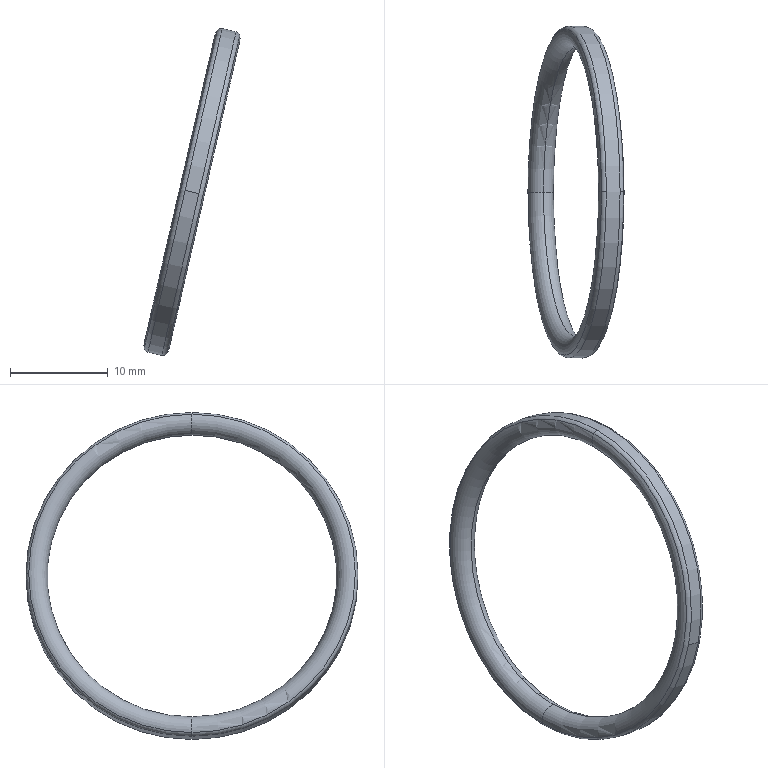Part | SolidWorks | features BaseBody 1 | 1 solid | 12 faces | box 9.855 x 34.04 x 33.526 mm | volume 478.172 mm3 | torus 10 | cylinder 2 | commonest cylinder face diameters 34.04 x2
STEP:
#1=CARTESIAN_POINT('',(1966.289,-176.,834.72));
#2=VERTEX_POINT('',#1);
#3=CARTESIAN_POINT('',(1964.722,-176.,833.139));
#4=VERTEX_POINT('',#3);
#5=CARTESIAN_POINT('',(1965.996,-176.,833.443));
#6=DIRECTION('',(0.,-1.,0.));
#7=DIRECTION('',(0.7736,0.,-0.6337));
#8=AXIS2_PLACEMENT_3D('',#5,#6,#7);
#9=CIRCLE('',#8,1.31);
#10=EDGE_CURVE('',#2,#4,#9,.T.);
#11=ORIENTED_EDGE('',*,*,#10,.F.);
#12=CARTESIAN_POINT('',(1972.938,-176.,863.666));
#13=VERTEX_POINT('',#12);
#14=CARTESIAN_POINT('',(1969.614,-176.,849.193));
#15=DIRECTION('',(0.9746,0.,-0.2239));
#16=DIRECTION('',(-0.2239,0.,-0.9746));
#17=AXIS2_PLACEMENT_3D('',#14,#15,#16);
#18=CIRCLE('',#17,14.85);
#19=EDGE_CURVE('',#2,#13,#18,.T.);
#20=ORIENTED_EDGE('',*,*,#19,.T.);
#21=CARTESIAN_POINT('',(1972.218,-176.,865.773));
#22=VERTEX_POINT('',#21);
#23=CARTESIAN_POINT('',(1973.231,-176.,864.943));
#24=DIRECTION('',(0.,-1.,0.));
#25=DIRECTION('',(-0.7736,0.,0.6337));
#26=AXIS2_PLACEMENT_3D('',#23,#24,#25);
#27=CIRCLE('',#26,1.31);
#28=EDGE_CURVE('',#22,#13,#27,.T.);
#29=ORIENTED_EDGE('',*,*,#28,.F.);
#30=CARTESIAN_POINT('',(1968.47,-159.258,849.456));
#31=VERTEX_POINT('',#30);
#32=CARTESIAN_POINT('',(1968.47,-176.,849.456));
#33=DIRECTION('',(-0.9746,0.,0.2239));
#34=DIRECTION('',(0.2239,0.,0.9746));
#35=AXIS2_PLACEMENT_3D('',#32,#33,#34);
#36=CIRCLE('',#35,16.742);
#37=EDGE_CURVE('',#22,#31,#36,.T.);
#38=ORIENTED_EDGE('',*,*,#37,.T.);
#39=CARTESIAN_POINT('',(1968.47,-176.,849.456));
#40=DIRECTION('',(-0.9746,0.,0.2239));
#41=DIRECTION('',(0.,1.,0.));
#42=AXIS2_PLACEMENT_3D('',#39,#40,#41);
#43=CIRCLE('',#42,16.742);
#44=EDGE_CURVE('',#31,#4,#43,.T.);
#45=ORIENTED_EDGE('',*,*,#44,.T.);
#46=EDGE_LOOP('',(#11,#20,#29,#38,#45));
#47=FACE_OUTER_BOUND('',#46,.T.);
#48=CARTESIAN_POINT('',(1969.614,-176.,849.193));
#49=DIRECTION('',(0.9746,0.,-0.2239));
#50=DIRECTION('',(0.2239,0.,0.9746));
#51=AXIS2_PLACEMENT_3D('',#48,#49,#50);
#52=TOROIDAL_SURFACE('',#51,16.16,1.31);
#53=ADVANCED_FACE('',(#47),#52,.T.);
#54=ORIENTED_EDGE('',*,*,#28,.T.);
#55=CARTESIAN_POINT('',(1969.614,-176.,849.193));
#56=DIRECTION('',(0.9746,0.,-0.2239));
#57=DIRECTION('',(-0.2239,0.,-0.9746));
#58=AXIS2_PLACEMENT_3D('',#55,#56,#57);
#59=CIRCLE('',#58,14.85);
#60=EDGE_CURVE('',#13,#2,#59,.T.);
#61=ORIENTED_EDGE('',*,*,#60,.T.);
#62=ORIENTED_EDGE('',*,*,#10,.T.);
#63=CARTESIAN_POINT('',(1968.47,-176.,849.456));
#64=DIRECTION('',(-0.9746,0.,0.2239));
#65=DIRECTION('',(-0.2239,0.,-0.9746));
#66=AXIS2_PLACEMENT_3D('',#63,#64,#65);
#67=CIRCLE('',#66,16.742);
#68=EDGE_CURVE('',#4,#22,#67,.T.);
#69=ORIENTED_EDGE('',*,*,#68,.T.);
#70=EDGE_LOOP('',(#54,#61,#62,#69));
#71=FACE_OUTER_BOUND('',#70,.T.);
#72=CARTESIAN_POINT('',(1969.614,-176.,849.193));
#73=DIRECTION('',(0.9746,0.,-0.2239));
#74=DIRECTION('',(0.2239,0.,0.9746));
#75=AXIS2_PLACEMENT_3D('',#72,#73,#74);
#76=TOROIDAL_SURFACE('',#75,16.16,1.31);
#77=ADVANCED_FACE('',(#71),#76,.T.);
#78=ORIENTED_EDGE('',*,*,#37,.F.);
#79=CARTESIAN_POINT('',(1972.716,-176.,865.944));
#80=VERTEX_POINT('',#79);
#81=CARTESIAN_POINT('',(1972.605,-176.,865.456));
#82=DIRECTION('',(0.,1.,0.));
#83=DIRECTION('',(-1.,0.,0.));
#84=AXIS2_PLACEMENT_3D('',#81,#82,#83);
#85=CIRCLE('',#84,0.5);
#86=EDGE_CURVE('',#22,#80,#85,.T.);
#87=ORIENTED_EDGE('',*,*,#86,.T.);
#88=CARTESIAN_POINT('',(1968.906,-158.98,849.356));
#89=VERTEX_POINT('',#88);
#90=CARTESIAN_POINT('',(1968.906,-176.,849.356));
#91=DIRECTION('',(0.9746,0.,-0.2239));
#92=DIRECTION('',(0.,1.,0.));
#93=AXIS2_PLACEMENT_3D('',#90,#91,#92);
#94=CIRCLE('',#93,17.02);
#95=EDGE_CURVE('',#89,#80,#94,.T.);
#96=ORIENTED_EDGE('',*,*,#95,.F.);
#97=CARTESIAN_POINT('',(1968.906,-159.48,849.356));
#98=DIRECTION('',(-0.2239,0.,-0.9746));
#99=DIRECTION('',(-0.8731,0.4444,0.2005));
#100=AXIS2_PLACEMENT_3D('',#97,#98,#99);
#101=CIRCLE('',#100,0.5);
#102=EDGE_CURVE('',#31,#89,#101,.T.);
#103=ORIENTED_EDGE('',*,*,#102,.F.);
#104=EDGE_LOOP('',(#78,#87,#96,#103));
#105=FACE_OUTER_BOUND('',#104,.T.);
#106=CARTESIAN_POINT('',(1968.906,-176.,849.356));
#107=DIRECTION('',(0.9746,0.,-0.2239));
#108=DIRECTION('',(0.2239,0.,0.9746));
#109=AXIS2_PLACEMENT_3D('',#106,#107,#108);
#110=TOROIDAL_SURFACE('',#109,16.52,0.5);
#111=ADVANCED_FACE('',(#105),#110,.T.);
#112=CARTESIAN_POINT('',(1974.131,-176.,865.619));
#113=VERTEX_POINT('',#112);
#114=CARTESIAN_POINT('',(1970.321,-158.98,849.031));
#115=VERTEX_POINT('',#114);
#116=CARTESIAN_POINT('',(1970.321,-176.,849.031));
#117=DIRECTION('',(-0.9746,0.,0.2239));
#118=DIRECTION('',(0.,-1.,0.));
#119=AXIS2_PLACEMENT_3D('',#116,#117,#118);
#120=CIRCLE('',#119,17.02);
#121=EDGE_CURVE('',#113,#115,#120,.T.);
#122=ORIENTED_EDGE('',*,*,#121,.F.);
#123=CARTESIAN_POINT('',(1974.505,-176.,865.248));
#124=VERTEX_POINT('',#123);
#125=CARTESIAN_POINT('',(1974.019,-176.,865.132));
#126=DIRECTION('',(0.,1.,0.));
#127=DIRECTION('',(-1.,0.,0.));
#128=AXIS2_PLACEMENT_3D('',#125,#126,#127);
#129=CIRCLE('',#128,0.5);
#130=EDGE_CURVE('',#113,#124,#129,.T.);
#131=ORIENTED_EDGE('',*,*,#130,.T.);
#132=CARTESIAN_POINT('',(1970.757,-159.258,848.931));
#133=VERTEX_POINT('',#132);
#134=CARTESIAN_POINT('',(1970.757,-176.,848.931));
#135=DIRECTION('',(0.9746,0.,-0.2239));
#136=DIRECTION('',(0.,1.,0.));
#137=AXIS2_PLACEMENT_3D('',#134,#135,#136);
#138=CIRCLE('',#137,16.742);
#139=EDGE_CURVE('',#133,#124,#138,.T.);
#140=ORIENTED_EDGE('',*,*,#139,.F.);
#141=CARTESIAN_POINT('',(1970.321,-159.48,849.031));
#142=DIRECTION('',(0.2239,0.,0.9746));
#143=DIRECTION('',(0.8731,0.4444,-0.2005));
#144=AXIS2_PLACEMENT_3D('',#141,#142,#143);
#145=CIRCLE('',#144,0.5);
#146=EDGE_CURVE('',#133,#115,#145,.T.);
#147=ORIENTED_EDGE('',*,*,#146,.T.);
#148=EDGE_LOOP('',(#122,#131,#140,#147));
#149=FACE_OUTER_BOUND('',#148,.T.);
#150=CARTESIAN_POINT('',(1970.321,-176.,849.031));
#151=DIRECTION('',(0.9746,0.,-0.2239));
#152=DIRECTION('',(0.2239,0.,0.9746));
#153=AXIS2_PLACEMENT_3D('',#150,#151,#152);
#154=TOROIDAL_SURFACE('',#153,16.52,0.5);
#155=ADVANCED_FACE('',(#149),#154,.T.);
#156=ORIENTED_EDGE('',*,*,#60,.F.);
#157=CARTESIAN_POINT('',(1973.231,-176.,864.943));
#158=DIRECTION('',(0.,-1.,0.));
#159=DIRECTION('',(-0.7736,0.,0.6337));
#160=AXIS2_PLACEMENT_3D('',#157,#158,#159);
#161=CIRCLE('',#160,1.31);
#162=EDGE_CURVE('',#13,#124,#161,.T.);
#163=ORIENTED_EDGE('',*,*,#162,.T.);
#164=CARTESIAN_POINT('',(1967.009,-176.,832.613));
#165=VERTEX_POINT('',#164);
#166=CARTESIAN_POINT('',(1970.757,-176.,848.931));
#167=DIRECTION('',(0.9746,0.,-0.2239));
#168=DIRECTION('',(0.2239,-0.000000033,0.9746));
#169=AXIS2_PLACEMENT_3D('',#166,#167,#168);
#170=CIRCLE('',#169,16.742);
#171=EDGE_CURVE('',#124,#165,#170,.T.);
#172=ORIENTED_EDGE('',*,*,#171,.T.);
#173=CARTESIAN_POINT('',(1965.996,-176.,833.443));
#174=DIRECTION('',(0.,-1.,0.));
#175=DIRECTION('',(0.7736,0.,-0.6337));
#176=AXIS2_PLACEMENT_3D('',#173,#174,#175);
#177=CIRCLE('',#176,1.31);
#178=EDGE_CURVE('',#165,#2,#177,.T.);
#179=ORIENTED_EDGE('',*,*,#178,.T.);
#180=EDGE_LOOP('',(#156,#163,#172,#179));
#181=FACE_OUTER_BOUND('',#180,.T.);
#182=CARTESIAN_POINT('',(1969.614,-176.,849.193));
#183=DIRECTION('',(0.9746,0.,-0.2239));
#184=DIRECTION('',(0.2239,0.,0.9746));
#185=AXIS2_PLACEMENT_3D('',#182,#183,#184);
#186=TOROIDAL_SURFACE('',#185,16.16,1.31);
#187=ADVANCED_FACE('',(#181),#186,.T.);
#188=ORIENTED_EDGE('',*,*,#130,.F.);
#189=CARTESIAN_POINT('',(1970.321,-193.02,849.031));
#190=VERTEX_POINT('',#189);
#191=CARTESIAN_POINT('',(1970.321,-176.,849.031));
#192=DIRECTION('',(-0.9746,0.,0.2239));
#193=DIRECTION('',(0.,-1.,0.));
#194=AXIS2_PLACEMENT_3D('',#191,#192,#193);
#195=CIRCLE('',#194,17.02);
#196=EDGE_CURVE('',#190,#113,#195,.T.);
#197=ORIENTED_EDGE('',*,*,#196,.F.);
#198=CARTESIAN_POINT('',(1966.511,-176.,832.443));
#199=VERTEX_POINT('',#198);
#200=CARTESIAN_POINT('',(1970.321,-176.,849.031));
#201=DIRECTION('',(0.9746,0.,-0.2239));
#202=DIRECTION('',(0.,-1.,0.));
#203=AXIS2_PLACEMENT_3D('',#200,#201,#202);
#204=CIRCLE('',#203,17.02);
#205=EDGE_CURVE('',#190,#199,#204,.T.);
#206=ORIENTED_EDGE('',*,*,#205,.T.);
#207=CARTESIAN_POINT('',(1966.622,-176.,832.93));
#208=DIRECTION('',(0.,-1.,0.));
#209=DIRECTION('',(0.7736,0.,-0.6337));
#210=AXIS2_PLACEMENT_3D('',#207,#208,#209);
#211=CIRCLE('',#210,0.5);
#212=EDGE_CURVE('',#199,#165,#211,.T.);
#213=ORIENTED_EDGE('',*,*,#212,.T.);
#214=ORIENTED_EDGE('',*,*,#171,.F.);
#215=EDGE_LOOP('',(#188,#197,#206,#213,#214));
#216=FACE_OUTER_BOUND('',#215,.T.);
#217=CARTESIAN_POINT('',(1970.321,-176.,849.031));
#218=DIRECTION('',(0.9746,0.,-0.2239));
#219=DIRECTION('',(0.2239,0.,0.9746));
#220=AXIS2_PLACEMENT_3D('',#217,#218,#219);
#221=TOROIDAL_SURFACE('',#220,16.52,0.5);
#222=ADVANCED_FACE('',(#216),#221,.T.);
#223=ORIENTED_EDGE('',*,*,#212,.F.);
#224=CARTESIAN_POINT('',(1970.321,-176.,849.031));
#225=DIRECTION('',(0.9746,0.,-0.2239));
#226=DIRECTION('',(-0.2239,-0.000000002,-0.9746));
#227=AXIS2_PLACEMENT_3D('',#224,#225,#226);
#228=CIRCLE('',#227,17.02);
#229=EDGE_CURVE('',#199,#115,#228,.T.);
#230=ORIENTED_EDGE('',*,*,#229,.T.);
#231=ORIENTED_EDGE('',*,*,#146,.F.);
#232=CARTESIAN_POINT('',(1970.757,-176.,848.931));
#233=DIRECTION('',(0.9746,0.,-0.2239));
#234=DIRECTION('',(-0.2239,0.,-0.9746));
#235=AXIS2_PLACEMENT_3D('',#232,#233,#234);
#236=CIRCLE('',#235,16.742);
#237=EDGE_CURVE('',#165,#133,#236,.T.);
#238=ORIENTED_EDGE('',*,*,#237,.F.);
#239=EDGE_LOOP('',(#223,#230,#231,#238));
#240=FACE_OUTER_BOUND('',#239,.T.);
#241=CARTESIAN_POINT('',(1970.321,-176.,849.031));
#242=DIRECTION('',(0.9746,0.,-0.2239));
#243=DIRECTION('',(0.2239,0.,0.9746));
#244=AXIS2_PLACEMENT_3D('',#241,#242,#243);
#245=TOROIDAL_SURFACE('',#244,16.52,0.5);
#246=ADVANCED_FACE('',(#240),#245,.T.);
#247=ORIENTED_EDGE('',*,*,#19,.F.);
#248=ORIENTED_EDGE('',*,*,#178,.F.);
#249=ORIENTED_EDGE('',*,*,#237,.T.);
#250=ORIENTED_EDGE('',*,*,#139,.T.);
#251=ORIENTED_EDGE('',*,*,#162,.F.);
#252=EDGE_LOOP('',(#247,#248,#249,#250,#251));
#253=FACE_OUTER_BOUND('',#252,.T.);
#254=CARTESIAN_POINT('',(1969.614,-176.,849.193));
#255=DIRECTION('',(0.9746,0.,-0.2239));
#256=DIRECTION('',(0.2239,0.,0.9746));
#257=AXIS2_PLACEMENT_3D('',#254,#255,#256);
#258=TOROIDAL_SURFACE('',#257,16.16,1.31);
#259=ADVANCED_FACE('',(#253),#258,.T.);
#260=ORIENTED_EDGE('',*,*,#102,.T.);
#261=CARTESIAN_POINT('',(1965.096,-176.,832.768));
#262=VERTEX_POINT('',#261);
#263=CARTESIAN_POINT('',(1968.906,-176.,849.356));
#264=DIRECTION('',(-0.9746,0.,0.2239));
#265=DIRECTION('',(0.,1.,0.));
#266=AXIS2_PLACEMENT_3D('',#263,#264,#265);
#267=CIRCLE('',#266,17.02);
#268=EDGE_CURVE('',#89,#262,#267,.T.);
#269=ORIENTED_EDGE('',*,*,#268,.T.);
#270=CARTESIAN_POINT('',(1965.208,-176.,833.255));
#271=DIRECTION('',(0.,1.,0.));
#272=DIRECTION('',(-0.9726,0.,-0.2326));
#273=AXIS2_PLACEMENT_3D('',#270,#271,#272);
#274=CIRCLE('',#273,0.5);
#275=EDGE_CURVE('',#262,#4,#274,.T.);
#276=ORIENTED_EDGE('',*,*,#275,.T.);
#277=ORIENTED_EDGE('',*,*,#44,.F.);
#278=EDGE_LOOP('',(#260,#269,#276,#277));
#279=FACE_OUTER_BOUND('',#278,.T.);
#280=CARTESIAN_POINT('',(1968.906,-176.,849.356));
#281=DIRECTION('',(0.9746,0.,-0.2239));
#282=DIRECTION('',(0.2239,0.,0.9746));
#283=AXIS2_PLACEMENT_3D('',#280,#281,#282);
#284=TOROIDAL_SURFACE('',#283,16.52,0.5);
#285=ADVANCED_FACE('',(#279),#284,.T.);
#286=ORIENTED_EDGE('',*,*,#86,.F.);
#287=ORIENTED_EDGE('',*,*,#68,.F.);
#288=ORIENTED_EDGE('',*,*,#275,.F.);
#289=CARTESIAN_POINT('',(1968.906,-193.02,849.356));
#290=VERTEX_POINT('',#289);
#291=CARTESIAN_POINT('',(1968.906,-176.,849.356));
#292=DIRECTION('',(-0.9746,0.,0.2239));
#293=DIRECTION('',(-0.2239,0.000000002,-0.9746));
#294=AXIS2_PLACEMENT_3D('',#291,#292,#293);
#295=CIRCLE('',#294,17.02);
#296=EDGE_CURVE('',#262,#290,#295,.T.);
#297=ORIENTED_EDGE('',*,*,#296,.T.);
#298=CARTESIAN_POINT('',(1968.906,-176.,849.356));
#299=DIRECTION('',(0.9746,0.,-0.2239));
#300=DIRECTION('',(0.,1.,0.));
#301=AXIS2_PLACEMENT_3D('',#298,#299,#300);
#302=CIRCLE('',#301,17.02);
#303=EDGE_CURVE('',#80,#290,#302,.T.);
#304=ORIENTED_EDGE('',*,*,#303,.F.);
#305=EDGE_LOOP('',(#286,#287,#288,#297,#304));
#306=FACE_OUTER_BOUND('',#305,.T.);
#307=CARTESIAN_POINT('',(1968.906,-176.,849.356));
#308=DIRECTION('',(0.9746,0.,-0.2239));
#309=DIRECTION('',(0.2239,0.,0.9746));
#310=AXIS2_PLACEMENT_3D('',#307,#308,#309);
#311=TOROIDAL_SURFACE('',#310,16.52,0.5);
#312=ADVANCED_FACE('',(#306),#311,.T.);
#313=CARTESIAN_POINT('',(1968.906,-158.98,849.356));
#314=DIRECTION('',(-0.9746,0.,0.2239));
#315=VECTOR('',#314,1000.);
#316=LINE('',#313,#315);
#317=EDGE_CURVE('',#115,#89,#316,.T.);
#318=ORIENTED_EDGE('',*,*,#317,.T.);
#319=ORIENTED_EDGE('',*,*,#95,.T.);
#320=ORIENTED_EDGE('',*,*,#303,.T.);
#321=CARTESIAN_POINT('',(1968.906,-193.02,849.356));
#322=DIRECTION('',(0.9746,0.,-0.2239));
#323=VECTOR('',#322,1000.);
#324=LINE('',#321,#323);
#325=EDGE_CURVE('',#290,#190,#324,.T.);
#326=ORIENTED_EDGE('',*,*,#325,.T.);
#327=ORIENTED_EDGE('',*,*,#196,.T.);
#328=ORIENTED_EDGE('',*,*,#121,.T.);
#329=EDGE_LOOP('',(#318,#319,#320,#326,#327,#328));
#330=FACE_OUTER_BOUND('',#329,.T.);
#331=CARTESIAN_POINT('',(1970.379,-176.,849.017));
#332=DIRECTION('',(-0.9746,0.,0.2239));
#333=DIRECTION('',(0.,1.,0.));
#334=AXIS2_PLACEMENT_3D('',#331,#332,#333);
#335=CYLINDRICAL_SURFACE('',#334,17.02);
#336=ADVANCED_FACE('',(#330),#335,.T.);
#337=ORIENTED_EDGE('',*,*,#325,.F.);
#338=ORIENTED_EDGE('',*,*,#296,.F.);
#339=ORIENTED_EDGE('',*,*,#268,.F.);
#340=ORIENTED_EDGE('',*,*,#317,.F.);
#341=ORIENTED_EDGE('',*,*,#229,.F.);
#342=ORIENTED_EDGE('',*,*,#205,.F.);
#343=EDGE_LOOP('',(#337,#338,#339,#340,#341,#342));
#344=FACE_OUTER_BOUND('',#343,.T.);
#345=CARTESIAN_POINT('',(1970.379,-176.,849.017));
#346=DIRECTION('',(-0.9746,0.,0.2239));
#347=DIRECTION('',(0.,1.,0.));
#348=AXIS2_PLACEMENT_3D('',#345,#346,#347);
#349=CYLINDRICAL_SURFACE('',#348,17.02);
#350=ADVANCED_FACE('',(#344),#349,.T.);
#351=CLOSED_SHELL('',(#53,#77,#111,#155,#187,#222,#246,#259,#285,#312,#336,#350));
#352=MANIFOLD_SOLID_BREP('',#351);
#353=CARTESIAN_POINT('',(0.,0.,0.));
#354=DIRECTION('',(0.,0.,1.));
#355=DIRECTION('',(1.,0.,0.));
#356=AXIS2_PLACEMENT_3D('',#353,#354,#355);
#357=(LENGTH_UNIT()NAMED_UNIT(*)SI_UNIT(.MILLI.,.METRE.));
#358=UNCERTAINTY_MEASURE_WITH_UNIT(LENGTH_MEASURE(0.00001),#357,'','');
#359=(NAMED_UNIT(*)PLANE_ANGLE_UNIT()SI_UNIT($,.RADIAN.));
#360=(NAMED_UNIT(*)SI_UNIT($,.STERADIAN.)SOLID_ANGLE_UNIT());
#361=(GEOMETRIC_REPRESENTATION_CONTEXT(3)GLOBAL_UNCERTAINTY_ASSIGNED_CONTEXT((#358))GLOBAL_UNIT_ASSIGNED_CONTEXT((#357,#359,#360))REPRESENTATION_CONTEXT('',''));
#362=ADVANCED_BREP_SHAPE_REPRESENTATION('',(#352,#356),#361);